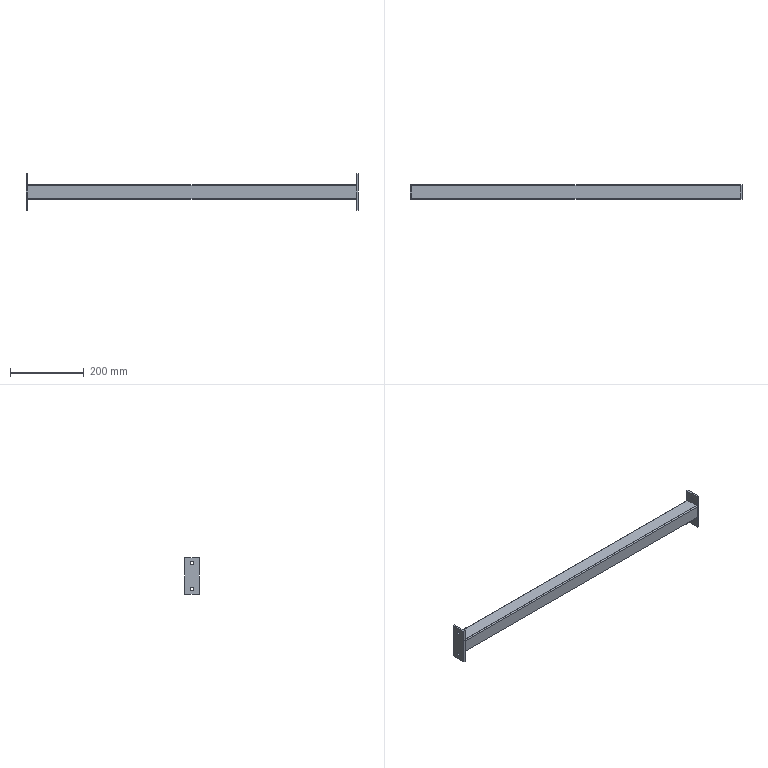Part | SolidWorks | features BaseBody 3 | 3 solids | 38 faces | box 897.45 x 40 x 100 mm | volume 238563 mm3 | plane 22 | cylinder 16 | commonest cylinder face diameters 9 x6 3 x4 6 x4 9.323 x2
STEP:
#1=CARTESIAN_POINT('',(0.,20.,17.));
#2=VERTEX_POINT('',#1);
#3=CARTESIAN_POINT('',(0.,17.,20.));
#4=VERTEX_POINT('',#3);
#5=CARTESIAN_POINT('',(0.,17.,17.));
#6=DIRECTION('',(1.,0.,0.));
#7=DIRECTION('',(0.,0.,-1.));
#8=AXIS2_PLACEMENT_3D('',#5,#6,#7);
#9=CIRCLE('',#8,3.);
#10=EDGE_CURVE('',#2,#4,#9,.T.);
#11=ORIENTED_EDGE('',*,*,#10,.T.);
#12=CARTESIAN_POINT('',(887.45,17.,20.));
#13=VERTEX_POINT('',#12);
#14=CARTESIAN_POINT('',(887.45,17.,20.));
#15=DIRECTION('',(-1.,0.,0.));
#16=VECTOR('',#15,1000.);
#17=LINE('',#14,#16);
#18=EDGE_CURVE('',#13,#4,#17,.T.);
#19=ORIENTED_EDGE('',*,*,#18,.F.);
#20=CARTESIAN_POINT('',(887.45,20.,17.));
#21=VERTEX_POINT('',#20);
#22=CARTESIAN_POINT('',(887.45,17.,17.));
#23=DIRECTION('',(1.,0.,0.));
#24=DIRECTION('',(0.,0.,-1.));
#25=AXIS2_PLACEMENT_3D('',#22,#23,#24);
#26=CIRCLE('',#25,3.);
#27=EDGE_CURVE('',#21,#13,#26,.T.);
#28=ORIENTED_EDGE('',*,*,#27,.F.);
#29=CARTESIAN_POINT('',(887.45,20.,17.));
#30=DIRECTION('',(-1.,0.,0.));
#31=VECTOR('',#30,1000.);
#32=LINE('',#29,#31);
#33=EDGE_CURVE('',#21,#2,#32,.T.);
#34=ORIENTED_EDGE('',*,*,#33,.T.);
#35=EDGE_LOOP('',(#11,#19,#28,#34));
#36=FACE_OUTER_BOUND('',#35,.T.);
#37=CARTESIAN_POINT('',(887.45,17.,17.));
#38=DIRECTION('',(-1.,0.,0.));
#39=DIRECTION('',(0.,0.,1.));
#40=AXIS2_PLACEMENT_3D('',#37,#38,#39);
#41=CYLINDRICAL_SURFACE('',#40,3.);
#42=ADVANCED_FACE('',(#36),#41,.T.);
#43=CARTESIAN_POINT('',(0.,-17.,20.));
#44=VERTEX_POINT('',#43);
#45=CARTESIAN_POINT('',(0.,17.,20.));
#46=DIRECTION('',(0.,-1.,0.));
#47=VECTOR('',#46,1000.);
#48=LINE('',#45,#47);
#49=EDGE_CURVE('',#4,#44,#48,.T.);
#50=ORIENTED_EDGE('',*,*,#49,.T.);
#51=CARTESIAN_POINT('',(887.45,-17.,20.));
#52=VERTEX_POINT('',#51);
#53=CARTESIAN_POINT('',(887.45,-17.,20.));
#54=DIRECTION('',(-1.,0.,0.));
#55=VECTOR('',#54,1000.);
#56=LINE('',#53,#55);
#57=EDGE_CURVE('',#52,#44,#56,.T.);
#58=ORIENTED_EDGE('',*,*,#57,.F.);
#59=CARTESIAN_POINT('',(887.45,17.,20.));
#60=DIRECTION('',(0.,-1.,0.));
#61=VECTOR('',#60,1000.);
#62=LINE('',#59,#61);
#63=EDGE_CURVE('',#13,#52,#62,.T.);
#64=ORIENTED_EDGE('',*,*,#63,.F.);
#65=ORIENTED_EDGE('',*,*,#18,.T.);
#66=EDGE_LOOP('',(#50,#58,#64,#65));
#67=FACE_OUTER_BOUND('',#66,.T.);
#68=CARTESIAN_POINT('',(887.45,17.,20.));
#69=DIRECTION('',(0.,0.,-1.));
#70=DIRECTION('',(0.,1.,0.));
#71=AXIS2_PLACEMENT_3D('',#68,#69,#70);
#72=PLANE('',#71);
#73=ADVANCED_FACE('',(#67),#72,.F.);
#74=CARTESIAN_POINT('',(0.,-20.,17.));
#75=VERTEX_POINT('',#74);
#76=CARTESIAN_POINT('',(0.,-17.,17.));
#77=DIRECTION('',(1.,0.,0.));
#78=DIRECTION('',(0.,0.,-1.));
#79=AXIS2_PLACEMENT_3D('',#76,#77,#78);
#80=CIRCLE('',#79,3.);
#81=EDGE_CURVE('',#44,#75,#80,.T.);
#82=ORIENTED_EDGE('',*,*,#81,.T.);
#83=CARTESIAN_POINT('',(887.45,-20.,17.));
#84=VERTEX_POINT('',#83);
#85=CARTESIAN_POINT('',(887.45,-20.,17.));
#86=DIRECTION('',(-1.,0.,0.));
#87=VECTOR('',#86,1000.);
#88=LINE('',#85,#87);
#89=EDGE_CURVE('',#84,#75,#88,.T.);
#90=ORIENTED_EDGE('',*,*,#89,.F.);
#91=CARTESIAN_POINT('',(887.45,-17.,17.));
#92=DIRECTION('',(1.,0.,0.));
#93=DIRECTION('',(0.,0.,-1.));
#94=AXIS2_PLACEMENT_3D('',#91,#92,#93);
#95=CIRCLE('',#94,3.);
#96=EDGE_CURVE('',#52,#84,#95,.T.);
#97=ORIENTED_EDGE('',*,*,#96,.F.);
#98=ORIENTED_EDGE('',*,*,#57,.T.);
#99=EDGE_LOOP('',(#82,#90,#97,#98));
#100=FACE_OUTER_BOUND('',#99,.T.);
#101=CARTESIAN_POINT('',(887.45,-17.,17.));
#102=DIRECTION('',(-1.,0.,0.));
#103=DIRECTION('',(0.,0.,1.));
#104=AXIS2_PLACEMENT_3D('',#101,#102,#103);
#105=CYLINDRICAL_SURFACE('',#104,3.);
#106=ADVANCED_FACE('',(#100),#105,.T.);
#107=CARTESIAN_POINT('',(0.,-20.,-17.));
#108=VERTEX_POINT('',#107);
#109=CARTESIAN_POINT('',(0.,-20.,-17.));
#110=DIRECTION('',(0.,0.,-1.));
#111=VECTOR('',#110,1000.);
#112=LINE('',#109,#111);
#113=EDGE_CURVE('',#75,#108,#112,.T.);
#114=ORIENTED_EDGE('',*,*,#113,.T.);
#115=CARTESIAN_POINT('',(887.45,-20.,-17.));
#116=VERTEX_POINT('',#115);
#117=CARTESIAN_POINT('',(887.45,-20.,-17.));
#118=DIRECTION('',(-1.,0.,0.));
#119=VECTOR('',#118,1000.);
#120=LINE('',#117,#119);
#121=EDGE_CURVE('',#116,#108,#120,.T.);
#122=ORIENTED_EDGE('',*,*,#121,.F.);
#123=CARTESIAN_POINT('',(887.45,-20.,-17.));
#124=DIRECTION('',(0.,0.,-1.));
#125=VECTOR('',#124,1000.);
#126=LINE('',#123,#125);
#127=EDGE_CURVE('',#84,#116,#126,.T.);
#128=ORIENTED_EDGE('',*,*,#127,.F.);
#129=ORIENTED_EDGE('',*,*,#89,.T.);
#130=EDGE_LOOP('',(#114,#122,#128,#129));
#131=FACE_OUTER_BOUND('',#130,.T.);
#132=CARTESIAN_POINT('',(887.45,-20.,-17.));
#133=DIRECTION('',(0.,1.,0.));
#134=DIRECTION('',(0.,0.,1.));
#135=AXIS2_PLACEMENT_3D('',#132,#133,#134);
#136=PLANE('',#135);
#137=ADVANCED_FACE('',(#131),#136,.F.);
#138=CARTESIAN_POINT('',(0.,-17.,-20.));
#139=VERTEX_POINT('',#138);
#140=CARTESIAN_POINT('',(0.,-17.,-17.));
#141=DIRECTION('',(1.,0.,0.));
#142=DIRECTION('',(0.,0.,-1.));
#143=AXIS2_PLACEMENT_3D('',#140,#141,#142);
#144=CIRCLE('',#143,3.);
#145=EDGE_CURVE('',#108,#139,#144,.T.);
#146=ORIENTED_EDGE('',*,*,#145,.T.);
#147=CARTESIAN_POINT('',(887.45,-17.,-20.));
#148=VERTEX_POINT('',#147);
#149=CARTESIAN_POINT('',(887.45,-17.,-20.));
#150=DIRECTION('',(-1.,0.,0.));
#151=VECTOR('',#150,1000.);
#152=LINE('',#149,#151);
#153=EDGE_CURVE('',#148,#139,#152,.T.);
#154=ORIENTED_EDGE('',*,*,#153,.F.);
#155=CARTESIAN_POINT('',(887.45,-17.,-17.));
#156=DIRECTION('',(1.,0.,0.));
#157=DIRECTION('',(0.,0.,-1.));
#158=AXIS2_PLACEMENT_3D('',#155,#156,#157);
#159=CIRCLE('',#158,3.);
#160=EDGE_CURVE('',#116,#148,#159,.T.);
#161=ORIENTED_EDGE('',*,*,#160,.F.);
#162=ORIENTED_EDGE('',*,*,#121,.T.);
#163=EDGE_LOOP('',(#146,#154,#161,#162));
#164=FACE_OUTER_BOUND('',#163,.T.);
#165=CARTESIAN_POINT('',(887.45,-17.,-17.));
#166=DIRECTION('',(-1.,0.,0.));
#167=DIRECTION('',(0.,0.,1.));
#168=AXIS2_PLACEMENT_3D('',#165,#166,#167);
#169=CYLINDRICAL_SURFACE('',#168,3.);
#170=ADVANCED_FACE('',(#164),#169,.T.);
#171=CARTESIAN_POINT('',(0.,17.,-20.));
#172=VERTEX_POINT('',#171);
#173=CARTESIAN_POINT('',(0.,-17.,-20.));
#174=DIRECTION('',(0.,1.,0.));
#175=VECTOR('',#174,1000.);
#176=LINE('',#173,#175);
#177=EDGE_CURVE('',#139,#172,#176,.T.);
#178=ORIENTED_EDGE('',*,*,#177,.T.);
#179=CARTESIAN_POINT('',(887.45,17.,-20.));
#180=VERTEX_POINT('',#179);
#181=CARTESIAN_POINT('',(887.45,17.,-20.));
#182=DIRECTION('',(-1.,0.,0.));
#183=VECTOR('',#182,1000.);
#184=LINE('',#181,#183);
#185=EDGE_CURVE('',#180,#172,#184,.T.);
#186=ORIENTED_EDGE('',*,*,#185,.F.);
#187=CARTESIAN_POINT('',(887.45,-17.,-20.));
#188=DIRECTION('',(0.,1.,0.));
#189=VECTOR('',#188,1000.);
#190=LINE('',#187,#189);
#191=EDGE_CURVE('',#148,#180,#190,.T.);
#192=ORIENTED_EDGE('',*,*,#191,.F.);
#193=ORIENTED_EDGE('',*,*,#153,.T.);
#194=EDGE_LOOP('',(#178,#186,#192,#193));
#195=FACE_OUTER_BOUND('',#194,.T.);
#196=CARTESIAN_POINT('',(887.45,-17.,-20.));
#197=DIRECTION('',(0.,0.,1.));
#198=DIRECTION('',(0.,-1.,0.));
#199=AXIS2_PLACEMENT_3D('',#196,#197,#198);
#200=PLANE('',#199);
#201=ADVANCED_FACE('',(#195),#200,.F.);
#202=CARTESIAN_POINT('',(0.,20.,-17.));
#203=VERTEX_POINT('',#202);
#204=CARTESIAN_POINT('',(0.,17.,-17.));
#205=DIRECTION('',(1.,0.,0.));
#206=DIRECTION('',(0.,0.,-1.));
#207=AXIS2_PLACEMENT_3D('',#204,#205,#206);
#208=CIRCLE('',#207,3.);
#209=EDGE_CURVE('',#172,#203,#208,.T.);
#210=ORIENTED_EDGE('',*,*,#209,.T.);
#211=CARTESIAN_POINT('',(887.45,20.,-17.));
#212=VERTEX_POINT('',#211);
#213=CARTESIAN_POINT('',(887.45,20.,-17.));
#214=DIRECTION('',(-1.,0.,0.));
#215=VECTOR('',#214,1000.);
#216=LINE('',#213,#215);
#217=EDGE_CURVE('',#212,#203,#216,.T.);
#218=ORIENTED_EDGE('',*,*,#217,.F.);
#219=CARTESIAN_POINT('',(887.45,17.,-17.));
#220=DIRECTION('',(1.,0.,0.));
#221=DIRECTION('',(0.,0.,-1.));
#222=AXIS2_PLACEMENT_3D('',#219,#220,#221);
#223=CIRCLE('',#222,3.);
#224=EDGE_CURVE('',#180,#212,#223,.T.);
#225=ORIENTED_EDGE('',*,*,#224,.F.);
#226=ORIENTED_EDGE('',*,*,#185,.T.);
#227=EDGE_LOOP('',(#210,#218,#225,#226));
#228=FACE_OUTER_BOUND('',#227,.T.);
#229=CARTESIAN_POINT('',(887.45,17.,-17.));
#230=DIRECTION('',(-1.,0.,0.));
#231=DIRECTION('',(0.,0.,1.));
#232=AXIS2_PLACEMENT_3D('',#229,#230,#231);
#233=CYLINDRICAL_SURFACE('',#232,3.);
#234=ADVANCED_FACE('',(#228),#233,.T.);
#235=CARTESIAN_POINT('',(0.,-17.,18.5));
#236=VERTEX_POINT('',#235);
#237=CARTESIAN_POINT('',(0.,-18.5,17.));
#238=VERTEX_POINT('',#237);
#239=CARTESIAN_POINT('',(0.,-17.,17.));
#240=DIRECTION('',(1.,0.,0.));
#241=DIRECTION('',(0.,0.,-1.));
#242=AXIS2_PLACEMENT_3D('',#239,#240,#241);
#243=CIRCLE('',#242,1.5);
#244=EDGE_CURVE('',#236,#238,#243,.T.);
#245=ORIENTED_EDGE('',*,*,#244,.F.);
#246=CARTESIAN_POINT('',(887.45,-17.,18.5));
#247=VERTEX_POINT('',#246);
#248=CARTESIAN_POINT('',(887.45,-17.,18.5));
#249=DIRECTION('',(-1.,0.,0.));
#250=VECTOR('',#249,1000.);
#251=LINE('',#248,#250);
#252=EDGE_CURVE('',#247,#236,#251,.T.);
#253=ORIENTED_EDGE('',*,*,#252,.F.);
#254=CARTESIAN_POINT('',(887.45,-18.5,17.));
#255=VERTEX_POINT('',#254);
#256=CARTESIAN_POINT('',(887.45,-17.,17.));
#257=DIRECTION('',(1.,0.,0.));
#258=DIRECTION('',(0.,0.,-1.));
#259=AXIS2_PLACEMENT_3D('',#256,#257,#258);
#260=CIRCLE('',#259,1.5);
#261=EDGE_CURVE('',#247,#255,#260,.T.);
#262=ORIENTED_EDGE('',*,*,#261,.T.);
#263=CARTESIAN_POINT('',(887.45,-18.5,17.));
#264=DIRECTION('',(-1.,0.,0.));
#265=VECTOR('',#264,1000.);
#266=LINE('',#263,#265);
#267=EDGE_CURVE('',#255,#238,#266,.T.);
#268=ORIENTED_EDGE('',*,*,#267,.T.);
#269=EDGE_LOOP('',(#245,#253,#262,#268));
#270=FACE_OUTER_BOUND('',#269,.T.);
#271=CARTESIAN_POINT('',(887.45,-17.,17.));
#272=DIRECTION('',(-1.,0.,0.));
#273=DIRECTION('',(0.,0.,1.));
#274=AXIS2_PLACEMENT_3D('',#271,#272,#273);
#275=CYLINDRICAL_SURFACE('',#274,1.5);
#276=ADVANCED_FACE('',(#270),#275,.F.);
#277=CARTESIAN_POINT('',(0.,17.,18.5));
#278=VERTEX_POINT('',#277);
#279=CARTESIAN_POINT('',(0.,17.,18.5));
#280=DIRECTION('',(0.,-1.,0.));
#281=VECTOR('',#280,1000.);
#282=LINE('',#279,#281);
#283=EDGE_CURVE('',#278,#236,#282,.T.);
#284=ORIENTED_EDGE('',*,*,#283,.F.);
#285=CARTESIAN_POINT('',(887.45,17.,18.5));
#286=VERTEX_POINT('',#285);
#287=CARTESIAN_POINT('',(887.45,17.,18.5));
#288=DIRECTION('',(-1.,0.,0.));
#289=VECTOR('',#288,1000.);
#290=LINE('',#287,#289);
#291=EDGE_CURVE('',#286,#278,#290,.T.);
#292=ORIENTED_EDGE('',*,*,#291,.F.);
#293=CARTESIAN_POINT('',(887.45,17.,18.5));
#294=DIRECTION('',(0.,-1.,0.));
#295=VECTOR('',#294,1000.);
#296=LINE('',#293,#295);
#297=EDGE_CURVE('',#286,#247,#296,.T.);
#298=ORIENTED_EDGE('',*,*,#297,.T.);
#299=ORIENTED_EDGE('',*,*,#252,.T.);
#300=EDGE_LOOP('',(#284,#292,#298,#299));
#301=FACE_OUTER_BOUND('',#300,.T.);
#302=CARTESIAN_POINT('',(887.45,17.,18.5));
#303=DIRECTION('',(0.,0.,-1.));
#304=DIRECTION('',(0.,1.,0.));
#305=AXIS2_PLACEMENT_3D('',#302,#303,#304);
#306=PLANE('',#305);
#307=ADVANCED_FACE('',(#301),#306,.T.);
#308=CARTESIAN_POINT('',(0.,18.5,17.));
#309=VERTEX_POINT('',#308);
#310=CARTESIAN_POINT('',(0.,17.,17.));
#311=DIRECTION('',(1.,0.,0.));
#312=DIRECTION('',(0.,0.,-1.));
#313=AXIS2_PLACEMENT_3D('',#310,#311,#312);
#314=CIRCLE('',#313,1.5);
#315=EDGE_CURVE('',#309,#278,#314,.T.);
#316=ORIENTED_EDGE('',*,*,#315,.F.);
#317=CARTESIAN_POINT('',(887.45,18.5,17.));
#318=VERTEX_POINT('',#317);
#319=CARTESIAN_POINT('',(887.45,18.5,17.));
#320=DIRECTION('',(-1.,0.,0.));
#321=VECTOR('',#320,1000.);
#322=LINE('',#319,#321);
#323=EDGE_CURVE('',#318,#309,#322,.T.);
#324=ORIENTED_EDGE('',*,*,#323,.F.);
#325=CARTESIAN_POINT('',(887.45,17.,17.));
#326=DIRECTION('',(1.,0.,0.));
#327=DIRECTION('',(0.,0.,-1.));
#328=AXIS2_PLACEMENT_3D('',#325,#326,#327);
#329=CIRCLE('',#328,1.5);
#330=EDGE_CURVE('',#318,#286,#329,.T.);
#331=ORIENTED_EDGE('',*,*,#330,.T.);
#332=ORIENTED_EDGE('',*,*,#291,.T.);
#333=EDGE_LOOP('',(#316,#324,#331,#332));
#334=FACE_OUTER_BOUND('',#333,.T.);
#335=CARTESIAN_POINT('',(887.45,17.,17.));
#336=DIRECTION('',(-1.,0.,0.));
#337=DIRECTION('',(0.,0.,1.));
#338=AXIS2_PLACEMENT_3D('',#335,#336,#337);
#339=CYLINDRICAL_SURFACE('',#338,1.5);
#340=ADVANCED_FACE('',(#334),#339,.F.);
#341=CARTESIAN_POINT('',(0.,18.5,-17.));
#342=VERTEX_POINT('',#341);
#343=CARTESIAN_POINT('',(0.,18.5,17.));
#344=DIRECTION('',(0.,0.,1.));
#345=VECTOR('',#344,1000.);
#346=LINE('',#343,#345);
#347=EDGE_CURVE('',#342,#309,#346,.T.);
#348=ORIENTED_EDGE('',*,*,#347,.F.);
#349=CARTESIAN_POINT('',(887.45,18.5,-17.));
#350=VERTEX_POINT('',#349);
#351=CARTESIAN_POINT('',(887.45,18.5,-17.));
#352=DIRECTION('',(-1.,0.,0.));
#353=VECTOR('',#352,1000.);
#354=LINE('',#351,#353);
#355=EDGE_CURVE('',#350,#342,#354,.T.);
#356=ORIENTED_EDGE('',*,*,#355,.F.);
#357=CARTESIAN_POINT('',(887.45,18.5,17.));
#358=DIRECTION('',(0.,0.,1.));
#359=VECTOR('',#358,1000.);
#360=LINE('',#357,#359);
#361=EDGE_CURVE('',#350,#318,#360,.T.);
#362=ORIENTED_EDGE('',*,*,#361,.T.);
#363=ORIENTED_EDGE('',*,*,#323,.T.);
#364=EDGE_LOOP('',(#348,#356,#362,#363));
#365=FACE_OUTER_BOUND('',#364,.T.);
#366=CARTESIAN_POINT('',(887.45,18.5,17.));
#367=DIRECTION('',(0.,-1.,0.));
#368=DIRECTION('',(0.,0.,-1.));
#369=AXIS2_PLACEMENT_3D('',#366,#367,#368);
#370=PLANE('',#369);
#371=ADVANCED_FACE('',(#365),#370,.T.);
#372=CARTESIAN_POINT('',(0.,17.,-18.5));
#373=VERTEX_POINT('',#372);
#374=CARTESIAN_POINT('',(0.,17.,-17.));
#375=DIRECTION('',(1.,0.,0.));
#376=DIRECTION('',(0.,0.,-1.));
#377=AXIS2_PLACEMENT_3D('',#374,#375,#376);
#378=CIRCLE('',#377,1.5);
#379=EDGE_CURVE('',#373,#342,#378,.T.);
#380=ORIENTED_EDGE('',*,*,#379,.F.);
#381=CARTESIAN_POINT('',(887.45,17.,-18.5));
#382=VERTEX_POINT('',#381);
#383=CARTESIAN_POINT('',(887.45,17.,-18.5));
#384=DIRECTION('',(-1.,0.,0.));
#385=VECTOR('',#384,1000.);
#386=LINE('',#383,#385);
#387=EDGE_CURVE('',#382,#373,#386,.T.);
#388=ORIENTED_EDGE('',*,*,#387,.F.);
#389=CARTESIAN_POINT('',(887.45,17.,-17.));
#390=DIRECTION('',(1.,0.,0.));
#391=DIRECTION('',(0.,0.,-1.));
#392=AXIS2_PLACEMENT_3D('',#389,#390,#391);
#393=CIRCLE('',#392,1.5);
#394=EDGE_CURVE('',#382,#350,#393,.T.);
#395=ORIENTED_EDGE('',*,*,#394,.T.);
#396=ORIENTED_EDGE('',*,*,#355,.T.);
#397=EDGE_LOOP('',(#380,#388,#395,#396));
#398=FACE_OUTER_BOUND('',#397,.T.);
#399=CARTESIAN_POINT('',(887.45,17.,-17.));
#400=DIRECTION('',(-1.,0.,0.));
#401=DIRECTION('',(0.,0.,1.));
#402=AXIS2_PLACEMENT_3D('',#399,#400,#401);
#403=CYLINDRICAL_SURFACE('',#402,1.5);
#404=ADVANCED_FACE('',(#398),#403,.F.);
#405=CARTESIAN_POINT('',(0.,-17.,-18.5));
#406=VERTEX_POINT('',#405);
#407=CARTESIAN_POINT('',(0.,-17.,-18.5));
#408=DIRECTION('',(0.,1.,0.));
#409=VECTOR('',#408,1000.);
#410=LINE('',#407,#409);
#411=EDGE_CURVE('',#406,#373,#410,.T.);
#412=ORIENTED_EDGE('',*,*,#411,.F.);
#413=CARTESIAN_POINT('',(887.45,-17.,-18.5));
#414=VERTEX_POINT('',#413);
#415=CARTESIAN_POINT('',(887.45,-17.,-18.5));
#416=DIRECTION('',(-1.,0.,0.));
#417=VECTOR('',#416,1000.);
#418=LINE('',#415,#417);
#419=EDGE_CURVE('',#414,#406,#418,.T.);
#420=ORIENTED_EDGE('',*,*,#419,.F.);
#421=CARTESIAN_POINT('',(887.45,-17.,-18.5));
#422=DIRECTION('',(0.,1.,0.));
#423=VECTOR('',#422,1000.);
#424=LINE('',#421,#423);
#425=EDGE_CURVE('',#414,#382,#424,.T.);
#426=ORIENTED_EDGE('',*,*,#425,.T.);
#427=ORIENTED_EDGE('',*,*,#387,.T.);
#428=EDGE_LOOP('',(#412,#420,#426,#427));
#429=FACE_OUTER_BOUND('',#428,.T.);
#430=CARTESIAN_POINT('',(887.45,-17.,-18.5));
#431=DIRECTION('',(0.,0.,1.));
#432=DIRECTION('',(0.,-1.,0.));
#433=AXIS2_PLACEMENT_3D('',#430,#431,#432);
#434=PLANE('',#433);
#435=ADVANCED_FACE('',(#429),#434,.T.);
#436=CARTESIAN_POINT('',(0.,-18.5,-17.));
#437=VERTEX_POINT('',#436);
#438=CARTESIAN_POINT('',(0.,-17.,-17.));
#439=DIRECTION('',(1.,0.,0.));
#440=DIRECTION('',(0.,0.,-1.));
#441=AXIS2_PLACEMENT_3D('',#438,#439,#440);
#442=CIRCLE('',#441,1.5);
#443=EDGE_CURVE('',#437,#406,#442,.T.);
#444=ORIENTED_EDGE('',*,*,#443,.F.);
#445=CARTESIAN_POINT('',(887.45,-18.5,-17.));
#446=VERTEX_POINT('',#445);
#447=CARTESIAN_POINT('',(887.45,-18.5,-17.));
#448=DIRECTION('',(-1.,0.,0.));
#449=VECTOR('',#448,1000.);
#450=LINE('',#447,#449);
#451=EDGE_CURVE('',#446,#437,#450,.T.);
#452=ORIENTED_EDGE('',*,*,#451,.F.);
#453=CARTESIAN_POINT('',(887.45,-17.,-17.));
#454=DIRECTION('',(1.,0.,0.));
#455=DIRECTION('',(0.,0.,-1.));
#456=AXIS2_PLACEMENT_3D('',#453,#454,#455);
#457=CIRCLE('',#456,1.5);
#458=EDGE_CURVE('',#446,#414,#457,.T.);
#459=ORIENTED_EDGE('',*,*,#458,.T.);
#460=ORIENTED_EDGE('',*,*,#419,.T.);
#461=EDGE_LOOP('',(#444,#452,#459,#460));
#462=FACE_OUTER_BOUND('',#461,.T.);
#463=CARTESIAN_POINT('',(887.45,-17.,-17.));
#464=DIRECTION('',(-1.,0.,0.));
#465=DIRECTION('',(0.,0.,1.));
#466=AXIS2_PLACEMENT_3D('',#463,#464,#465);
#467=CYLINDRICAL_SURFACE('',#466,1.5);
#468=ADVANCED_FACE('',(#462),#467,.F.);
#469=CARTESIAN_POINT('',(0.,-18.5,-17.));
#470=DIRECTION('',(0.,0.,-1.));
#471=VECTOR('',#470,1000.);
#472=LINE('',#469,#471);
#473=EDGE_CURVE('',#238,#437,#472,.T.);
#474=ORIENTED_EDGE('',*,*,#473,.F.);
#475=ORIENTED_EDGE('',*,*,#267,.F.);
#476=CARTESIAN_POINT('',(887.45,-18.5,-17.));
#477=DIRECTION('',(0.,0.,-1.));
#478=VECTOR('',#477,1000.);
#479=LINE('',#476,#478);
#480=EDGE_CURVE('',#255,#446,#479,.T.);
#481=ORIENTED_EDGE('',*,*,#480,.T.);
#482=ORIENTED_EDGE('',*,*,#451,.T.);
#483=EDGE_LOOP('',(#474,#475,#481,#482));
#484=FACE_OUTER_BOUND('',#483,.T.);
#485=CARTESIAN_POINT('',(887.45,-18.5,-17.));
#486=DIRECTION('',(0.,1.,0.));
#487=DIRECTION('',(0.,0.,1.));
#488=AXIS2_PLACEMENT_3D('',#485,#486,#487);
#489=PLANE('',#488);
#490=ADVANCED_FACE('',(#484),#489,.T.);
#491=CARTESIAN_POINT('',(0.,20.,17.));
#492=DIRECTION('',(0.,0.,1.));
#493=VECTOR('',#492,1000.);
#494=LINE('',#491,#493);
#495=EDGE_CURVE('',#203,#2,#494,.T.);
#496=ORIENTED_EDGE('',*,*,#495,.T.);
#497=ORIENTED_EDGE('',*,*,#33,.F.);
#498=CARTESIAN_POINT('',(887.45,20.,17.));
#499=DIRECTION('',(0.,0.,1.));
#500=VECTOR('',#499,1000.);
#501=LINE('',#498,#500);
#502=EDGE_CURVE('',#212,#21,#501,.T.);
#503=ORIENTED_EDGE('',*,*,#502,.F.);
#504=ORIENTED_EDGE('',*,*,#217,.T.);
#505=EDGE_LOOP('',(#496,#497,#503,#504));
#506=FACE_OUTER_BOUND('',#505,.T.);
#507=CARTESIAN_POINT('',(887.45,20.,17.));
#508=DIRECTION('',(0.,-1.,0.));
#509=DIRECTION('',(0.,0.,-1.));
#510=AXIS2_PLACEMENT_3D('',#507,#508,#509);
#511=PLANE('',#510);
#512=ADVANCED_FACE('',(#506),#511,.F.);
#513=ORIENTED_EDGE('',*,*,#261,.F.);
#514=ORIENTED_EDGE('',*,*,#297,.F.);
#515=ORIENTED_EDGE('',*,*,#330,.F.);
#516=ORIENTED_EDGE('',*,*,#361,.F.);
#517=ORIENTED_EDGE('',*,*,#394,.F.);
#518=ORIENTED_EDGE('',*,*,#425,.F.);
#519=ORIENTED_EDGE('',*,*,#458,.F.);
#520=ORIENTED_EDGE('',*,*,#480,.F.);
#521=EDGE_LOOP('',(#513,#514,#515,#516,#517,#518,#519,#520));
#522=FACE_BOUND('',#521,.T.);
#523=ORIENTED_EDGE('',*,*,#27,.T.);
#524=ORIENTED_EDGE('',*,*,#63,.T.);
#525=ORIENTED_EDGE('',*,*,#96,.T.);
#526=ORIENTED_EDGE('',*,*,#127,.T.);
#527=ORIENTED_EDGE('',*,*,#160,.T.);
#528=ORIENTED_EDGE('',*,*,#191,.T.);
#529=ORIENTED_EDGE('',*,*,#224,.T.);
#530=ORIENTED_EDGE('',*,*,#502,.T.);
#531=EDGE_LOOP('',(#523,#524,#525,#526,#527,#528,#529,#530));
#532=FACE_OUTER_BOUND('',#531,.T.);
#533=CARTESIAN_POINT('',(887.45,17.,17.));
#534=DIRECTION('',(1.,0.,0.));
#535=DIRECTION('',(0.,0.,-1.));
#536=AXIS2_PLACEMENT_3D('',#533,#534,#535);
#537=PLANE('',#536);
#538=ADVANCED_FACE('',(#522,#532),#537,.T.);
#539=ORIENTED_EDGE('',*,*,#244,.T.);
#540=ORIENTED_EDGE('',*,*,#473,.T.);
#541=ORIENTED_EDGE('',*,*,#443,.T.);
#542=ORIENTED_EDGE('',*,*,#411,.T.);
#543=ORIENTED_EDGE('',*,*,#379,.T.);
#544=ORIENTED_EDGE('',*,*,#347,.T.);
#545=ORIENTED_EDGE('',*,*,#315,.T.);
#546=ORIENTED_EDGE('',*,*,#283,.T.);
#547=EDGE_LOOP('',(#539,#540,#541,#542,#543,#544,#545,#546));
#548=FACE_BOUND('',#547,.T.);
#549=ORIENTED_EDGE('',*,*,#10,.F.);
#550=ORIENTED_EDGE('',*,*,#495,.F.);
#551=ORIENTED_EDGE('',*,*,#209,.F.);
#552=ORIENTED_EDGE('',*,*,#177,.F.);
#553=ORIENTED_EDGE('',*,*,#145,.F.);
#554=ORIENTED_EDGE('',*,*,#113,.F.);
#555=ORIENTED_EDGE('',*,*,#81,.F.);
#556=ORIENTED_EDGE('',*,*,#49,.F.);
#557=EDGE_LOOP('',(#549,#550,#551,#552,#553,#554,#555,#556));
#558=FACE_OUTER_BOUND('',#557,.T.);
#559=CARTESIAN_POINT('',(0.,17.,17.));
#560=DIRECTION('',(1.,0.,0.));
#561=DIRECTION('',(0.,0.,-1.));
#562=AXIS2_PLACEMENT_3D('',#559,#560,#561);
#563=PLANE('',#562);
#564=ADVANCED_FACE('',(#548,#558),#563,.F.);
#565=CLOSED_SHELL('',(#42,#73,#106,#137,#170,#201,#234,#276,#307,#340,#371,#404,#435,#468,#490,#512,#538,#564));
#566=MANIFOLD_SOLID_BREP('',#565);
#567=CARTESIAN_POINT('',(892.45,0.,39.5));
#568=VERTEX_POINT('',#567);
#569=CARTESIAN_POINT('',(892.45,0.,30.5));
#570=VERTEX_POINT('',#569);
#571=CARTESIAN_POINT('',(892.45,0.,35.));
#572=DIRECTION('',(1.,0.,0.));
#573=DIRECTION('',(0.,0.,-1.));
#574=AXIS2_PLACEMENT_3D('',#571,#572,#573);
#575=CIRCLE('',#574,4.5);
#576=EDGE_CURVE('',#568,#570,#575,.T.);
#577=ORIENTED_EDGE('',*,*,#576,.T.);
#578=CARTESIAN_POINT('',(887.45,0.,30.5));
#579=VERTEX_POINT('',#578);
#580=CARTESIAN_POINT('',(892.45,0.,30.5));
#581=DIRECTION('',(-1.,0.,0.));
#582=VECTOR('',#581,1000.);
#583=LINE('',#580,#582);
#584=EDGE_CURVE('',#570,#579,#583,.T.);
#585=ORIENTED_EDGE('',*,*,#584,.T.);
#586=CARTESIAN_POINT('',(887.45,0.,39.5));
#587=VERTEX_POINT('',#586);
#588=CARTESIAN_POINT('',(887.45,0.,35.));
#589=DIRECTION('',(1.,0.,0.));
#590=DIRECTION('',(0.,0.,-1.));
#591=AXIS2_PLACEMENT_3D('',#588,#589,#590);
#592=CIRCLE('',#591,4.5);
#593=EDGE_CURVE('',#587,#579,#592,.T.);
#594=ORIENTED_EDGE('',*,*,#593,.F.);
#595=CARTESIAN_POINT('',(892.45,0.,39.5));
#596=DIRECTION('',(-1.,0.,0.));
#597=VECTOR('',#596,1000.);
#598=LINE('',#595,#597);
#599=EDGE_CURVE('',#568,#587,#598,.T.);
#600=ORIENTED_EDGE('',*,*,#599,.F.);
#601=EDGE_LOOP('',(#577,#585,#594,#600));
#602=FACE_OUTER_BOUND('',#601,.T.);
#603=CARTESIAN_POINT('',(892.45,0.,35.));
#604=DIRECTION('',(-1.,0.,0.));
#605=DIRECTION('',(0.,0.,1.));
#606=AXIS2_PLACEMENT_3D('',#603,#604,#605);
#607=CYLINDRICAL_SURFACE('',#606,4.5);
#608=ADVANCED_FACE('',(#602),#607,.F.);
#609=CARTESIAN_POINT('',(892.45,0.,-30.5));
#610=VERTEX_POINT('',#609);
#611=CARTESIAN_POINT('',(892.45,0.,-39.5));
#612=VERTEX_POINT('',#611);
#613=CARTESIAN_POINT('',(892.45,0.,-35.));
#614=DIRECTION('',(1.,0.,0.));
#615=DIRECTION('',(0.,0.,-1.));
#616=AXIS2_PLACEMENT_3D('',#613,#614,#615);
#617=CIRCLE('',#616,4.5);
#618=EDGE_CURVE('',#610,#612,#617,.T.);
#619=ORIENTED_EDGE('',*,*,#618,.T.);
#620=CARTESIAN_POINT('',(887.45,0.,-39.5));
#621=VERTEX_POINT('',#620);
#622=CARTESIAN_POINT('',(892.45,0.,-39.5));
#623=DIRECTION('',(-1.,0.,0.));
#624=VECTOR('',#623,1000.);
#625=LINE('',#622,#624);
#626=EDGE_CURVE('',#612,#621,#625,.T.);
#627=ORIENTED_EDGE('',*,*,#626,.T.);
#628=CARTESIAN_POINT('',(887.45,0.,-30.5));
#629=VERTEX_POINT('',#628);
#630=CARTESIAN_POINT('',(887.45,0.,-35.));
#631=DIRECTION('',(1.,0.,0.));
#632=DIRECTION('',(0.,0.,-1.));
#633=AXIS2_PLACEMENT_3D('',#630,#631,#632);
#634=CIRCLE('',#633,4.5);
#635=EDGE_CURVE('',#629,#621,#634,.T.);
#636=ORIENTED_EDGE('',*,*,#635,.F.);
#637=CARTESIAN_POINT('',(892.45,0.,-30.5));
#638=DIRECTION('',(-1.,0.,0.));
#639=VECTOR('',#638,1000.);
#640=LINE('',#637,#639);
#641=EDGE_CURVE('',#610,#629,#640,.T.);
#642=ORIENTED_EDGE('',*,*,#641,.F.);
#643=EDGE_LOOP('',(#619,#627,#636,#642));
#644=FACE_OUTER_BOUND('',#643,.T.);
#645=CARTESIAN_POINT('',(892.45,0.,-35.));
#646=DIRECTION('',(-1.,0.,0.));
#647=DIRECTION('',(0.,0.,1.));
#648=AXIS2_PLACEMENT_3D('',#645,#646,#647);
#649=CYLINDRICAL_SURFACE('',#648,4.5);
#650=ADVANCED_FACE('',(#644),#649,.F.);
#651=CARTESIAN_POINT('',(892.45,-20.,-50.));
#652=VERTEX_POINT('',#651);
#653=CARTESIAN_POINT('',(892.45,20.,-50.));
#654=VERTEX_POINT('',#653);
#655=CARTESIAN_POINT('',(892.45,-20.,-50.));
#656=DIRECTION('',(0.,1.,0.));
#657=VECTOR('',#656,1000.);
#658=LINE('',#655,#657);
#659=EDGE_CURVE('',#652,#654,#658,.T.);
#660=ORIENTED_EDGE('',*,*,#659,.T.);
#661=CARTESIAN_POINT('',(892.45,20.,50.));
#662=VERTEX_POINT('',#661);
#663=CARTESIAN_POINT('',(892.45,20.,50.));
#664=DIRECTION('',(0.,0.,1.));
#665=VECTOR('',#664,1000.);
#666=LINE('',#663,#665);
#667=EDGE_CURVE('',#654,#662,#666,.T.);
#668=ORIENTED_EDGE('',*,*,#667,.T.);
#669=CARTESIAN_POINT('',(892.45,-20.,50.));
#670=VERTEX_POINT('',#669);
#671=CARTESIAN_POINT('',(892.45,-20.,50.));
#672=DIRECTION('',(0.,-1.,0.));
#673=VECTOR('',#672,1000.);
#674=LINE('',#671,#673);
#675=EDGE_CURVE('',#662,#670,#674,.T.);
#676=ORIENTED_EDGE('',*,*,#675,.T.);
#677=CARTESIAN_POINT('',(892.45,-20.,50.));
#678=DIRECTION('',(0.,0.,-1.));
#679=VECTOR('',#678,1000.);
#680=LINE('',#677,#679);
#681=EDGE_CURVE('',#670,#652,#680,.T.);
#682=ORIENTED_EDGE('',*,*,#681,.T.);
#683=EDGE_LOOP('',(#660,#668,#676,#682));
#684=FACE_OUTER_BOUND('',#683,.T.);
#685=ORIENTED_EDGE('',*,*,#618,.F.);
#686=CARTESIAN_POINT('',(892.45,0.,-35.));
#687=DIRECTION('',(1.,0.,0.));
#688=DIRECTION('',(0.,0.,-1.));
#689=AXIS2_PLACEMENT_3D('',#686,#687,#688);
#690=CIRCLE('',#689,4.5);
#691=EDGE_CURVE('',#612,#610,#690,.T.);
#692=ORIENTED_EDGE('',*,*,#691,.F.);
#693=EDGE_LOOP('',(#685,#692));
#694=FACE_BOUND('',#693,.T.);
#695=ORIENTED_EDGE('',*,*,#576,.F.);
#696=CARTESIAN_POINT('',(892.45,0.,35.));
#697=DIRECTION('',(1.,0.,0.));
#698=DIRECTION('',(0.,0.,-1.));
#699=AXIS2_PLACEMENT_3D('',#696,#697,#698);
#700=CIRCLE('',#699,4.5);
#701=EDGE_CURVE('',#570,#568,#700,.T.);
#702=ORIENTED_EDGE('',*,*,#701,.F.);
#703=EDGE_LOOP('',(#695,#702));
#704=FACE_BOUND('',#703,.T.);
#705=CARTESIAN_POINT('',(892.45,0.,0.));
#706=DIRECTION('',(-1.,0.,0.));
#707=DIRECTION('',(0.,0.,1.));
#708=AXIS2_PLACEMENT_3D('',#705,#706,#707);
#709=PLANE('',#708);
#710=ADVANCED_FACE('',(#684,#694,#704),#709,.F.);
#711=ORIENTED_EDGE('',*,*,#635,.T.);
#712=CARTESIAN_POINT('',(887.45,0.,-35.));
#713=DIRECTION('',(1.,0.,0.));
#714=DIRECTION('',(0.,0.,-1.));
#715=AXIS2_PLACEMENT_3D('',#712,#713,#714);
#716=CIRCLE('',#715,4.5);
#717=EDGE_CURVE('',#621,#629,#716,.T.);
#718=ORIENTED_EDGE('',*,*,#717,.T.);
#719=EDGE_LOOP('',(#711,#718));
#720=FACE_BOUND('',#719,.T.);
#721=CARTESIAN_POINT('',(887.45,-20.,-50.));
#722=VERTEX_POINT('',#721);
#723=CARTESIAN_POINT('',(887.45,20.,-50.));
#724=VERTEX_POINT('',#723);
#725=CARTESIAN_POINT('',(887.45,-20.,-50.));
#726=DIRECTION('',(0.,1.,0.));
#727=VECTOR('',#726,1000.);
#728=LINE('',#725,#727);
#729=EDGE_CURVE('',#722,#724,#728,.T.);
#730=ORIENTED_EDGE('',*,*,#729,.F.);
#731=CARTESIAN_POINT('',(887.45,-20.,50.));
#732=VERTEX_POINT('',#731);
#733=CARTESIAN_POINT('',(887.45,-20.,50.));
#734=DIRECTION('',(0.,0.,-1.));
#735=VECTOR('',#734,1000.);
#736=LINE('',#733,#735);
#737=EDGE_CURVE('',#732,#722,#736,.T.);
#738=ORIENTED_EDGE('',*,*,#737,.F.);
#739=CARTESIAN_POINT('',(887.45,20.,50.));
#740=VERTEX_POINT('',#739);
#741=CARTESIAN_POINT('',(887.45,-20.,50.));
#742=DIRECTION('',(0.,-1.,0.));
#743=VECTOR('',#742,1000.);
#744=LINE('',#741,#743);
#745=EDGE_CURVE('',#740,#732,#744,.T.);
#746=ORIENTED_EDGE('',*,*,#745,.F.);
#747=CARTESIAN_POINT('',(887.45,20.,50.));
#748=DIRECTION('',(0.,0.,1.));
#749=VECTOR('',#748,1000.);
#750=LINE('',#747,#749);
#751=EDGE_CURVE('',#724,#740,#750,.T.);
#752=ORIENTED_EDGE('',*,*,#751,.F.);
#753=EDGE_LOOP('',(#730,#738,#746,#752));
#754=FACE_OUTER_BOUND('',#753,.T.);
#755=ORIENTED_EDGE('',*,*,#593,.T.);
#756=CARTESIAN_POINT('',(887.45,0.,35.));
#757=DIRECTION('',(1.,0.,0.));
#758=DIRECTION('',(0.,0.,-1.));
#759=AXIS2_PLACEMENT_3D('',#756,#757,#758);
#760=CIRCLE('',#759,4.5);
#761=EDGE_CURVE('',#579,#587,#760,.T.);
#762=ORIENTED_EDGE('',*,*,#761,.T.);
#763=EDGE_LOOP('',(#755,#762));
#764=FACE_BOUND('',#763,.T.);
#765=CARTESIAN_POINT('',(887.45,0.,0.));
#766=DIRECTION('',(-1.,0.,0.));
#767=DIRECTION('',(0.,0.,1.));
#768=AXIS2_PLACEMENT_3D('',#765,#766,#767);
#769=PLANE('',#768);
#770=ADVANCED_FACE('',(#720,#754,#764),#769,.T.);
#771=ORIENTED_EDGE('',*,*,#729,.T.);
#772=CARTESIAN_POINT('',(892.45,20.,-50.));
#773=DIRECTION('',(-1.,0.,0.));
#774=VECTOR('',#773,1000.);
#775=LINE('',#772,#774);
#776=EDGE_CURVE('',#654,#724,#775,.T.);
#777=ORIENTED_EDGE('',*,*,#776,.F.);
#778=ORIENTED_EDGE('',*,*,#659,.F.);
#779=CARTESIAN_POINT('',(892.45,-20.,-50.));
#780=DIRECTION('',(-1.,0.,0.));
#781=VECTOR('',#780,1000.);
#782=LINE('',#779,#781);
#783=EDGE_CURVE('',#652,#722,#782,.T.);
#784=ORIENTED_EDGE('',*,*,#783,.T.);
#785=EDGE_LOOP('',(#771,#777,#778,#784));
#786=FACE_OUTER_BOUND('',#785,.T.);
#787=CARTESIAN_POINT('',(892.45,-20.,-50.));
#788=DIRECTION('',(0.,0.,1.));
#789=DIRECTION('',(1.,0.,0.));
#790=AXIS2_PLACEMENT_3D('',#787,#788,#789);
#791=PLANE('',#790);
#792=ADVANCED_FACE('',(#786),#791,.F.);
#793=ORIENTED_EDGE('',*,*,#751,.T.);
#794=CARTESIAN_POINT('',(892.45,20.,50.));
#795=DIRECTION('',(-1.,0.,0.));
#796=VECTOR('',#795,1000.);
#797=LINE('',#794,#796);
#798=EDGE_CURVE('',#662,#740,#797,.T.);
#799=ORIENTED_EDGE('',*,*,#798,.F.);
#800=ORIENTED_EDGE('',*,*,#667,.F.);
#801=ORIENTED_EDGE('',*,*,#776,.T.);
#802=EDGE_LOOP('',(#793,#799,#800,#801));
#803=FACE_OUTER_BOUND('',#802,.T.);
#804=CARTESIAN_POINT('',(892.45,20.,50.));
#805=DIRECTION('',(0.,-1.,0.));
#806=DIRECTION('',(0.,0.,-1.));
#807=AXIS2_PLACEMENT_3D('',#804,#805,#806);
#808=PLANE('',#807);
#809=ADVANCED_FACE('',(#803),#808,.F.);
#810=ORIENTED_EDGE('',*,*,#745,.T.);
#811=CARTESIAN_POINT('',(892.45,-20.,50.));
#812=DIRECTION('',(-1.,0.,0.));
#813=VECTOR('',#812,1000.);
#814=LINE('',#811,#813);
#815=EDGE_CURVE('',#670,#732,#814,.T.);
#816=ORIENTED_EDGE('',*,*,#815,.F.);
#817=ORIENTED_EDGE('',*,*,#675,.F.);
#818=ORIENTED_EDGE('',*,*,#798,.T.);
#819=EDGE_LOOP('',(#810,#816,#817,#818));
#820=FACE_OUTER_BOUND('',#819,.T.);
#821=CARTESIAN_POINT('',(892.45,-20.,50.));
#822=DIRECTION('',(0.,0.,-1.));
#823=DIRECTION('',(-1.,0.,0.));
#824=AXIS2_PLACEMENT_3D('',#821,#822,#823);
#825=PLANE('',#824);
#826=ADVANCED_FACE('',(#820),#825,.F.);
#827=ORIENTED_EDGE('',*,*,#737,.T.);
#828=ORIENTED_EDGE('',*,*,#783,.F.);
#829=ORIENTED_EDGE('',*,*,#681,.F.);
#830=ORIENTED_EDGE('',*,*,#815,.T.);
#831=EDGE_LOOP('',(#827,#828,#829,#830));
#832=FACE_OUTER_BOUND('',#831,.T.);
#833=CARTESIAN_POINT('',(892.45,-20.,50.));
#834=DIRECTION('',(0.,1.,0.));
#835=DIRECTION('',(0.,0.,1.));
#836=AXIS2_PLACEMENT_3D('',#833,#834,#835);
#837=PLANE('',#836);
#838=ADVANCED_FACE('',(#832),#837,.F.);
#839=ORIENTED_EDGE('',*,*,#626,.F.);
#840=ORIENTED_EDGE('',*,*,#691,.T.);
#841=ORIENTED_EDGE('',*,*,#641,.T.);
#842=ORIENTED_EDGE('',*,*,#717,.F.);
#843=EDGE_LOOP('',(#839,#840,#841,#842));
#844=FACE_OUTER_BOUND('',#843,.T.);
#845=CARTESIAN_POINT('',(892.45,0.,-35.));
#846=DIRECTION('',(-1.,0.,0.));
#847=DIRECTION('',(0.,0.,1.));
#848=AXIS2_PLACEMENT_3D('',#845,#846,#847);
#849=CYLINDRICAL_SURFACE('',#848,4.5);
#850=ADVANCED_FACE('',(#844),#849,.F.);
#851=ORIENTED_EDGE('',*,*,#584,.F.);
#852=ORIENTED_EDGE('',*,*,#701,.T.);
#853=ORIENTED_EDGE('',*,*,#599,.T.);
#854=ORIENTED_EDGE('',*,*,#761,.F.);
#855=EDGE_LOOP('',(#851,#852,#853,#854));
#856=FACE_OUTER_BOUND('',#855,.T.);
#857=CARTESIAN_POINT('',(892.45,0.,35.));
#858=DIRECTION('',(-1.,0.,0.));
#859=DIRECTION('',(0.,0.,1.));
#860=AXIS2_PLACEMENT_3D('',#857,#858,#859);
#861=CYLINDRICAL_SURFACE('',#860,4.5);
#862=ADVANCED_FACE('',(#856),#861,.F.);
#863=CLOSED_SHELL('',(#608,#650,#710,#770,#792,#809,#826,#838,#850,#862));
#864=MANIFOLD_SOLID_BREP('',#863);
#865=CARTESIAN_POINT('',(-5.,0.,-39.5));
#866=VERTEX_POINT('',#865);
#867=CARTESIAN_POINT('',(-5.,0.,-30.5));
#868=VERTEX_POINT('',#867);
#869=CARTESIAN_POINT('',(-5.,0.,-35.));
#870=DIRECTION('',(-1.,0.,0.));
#871=DIRECTION('',(0.,0.,1.));
#872=AXIS2_PLACEMENT_3D('',#869,#870,#871);
#873=CIRCLE('',#872,4.5);
#874=EDGE_CURVE('',#866,#868,#873,.T.);
#875=ORIENTED_EDGE('',*,*,#874,.T.);
#876=CARTESIAN_POINT('',(0.,0.,-30.5));
#877=VERTEX_POINT('',#876);
#878=CARTESIAN_POINT('',(-5.,0.,-30.5));
#879=DIRECTION('',(1.,0.,0.));
#880=VECTOR('',#879,1000.);
#881=LINE('',#878,#880);
#882=EDGE_CURVE('',#868,#877,#881,.T.);
#883=ORIENTED_EDGE('',*,*,#882,.T.);
#884=CARTESIAN_POINT('',(0.,0.,-39.5));
#885=VERTEX_POINT('',#884);
#886=CARTESIAN_POINT('',(0.,0.,-35.));
#887=DIRECTION('',(-1.,0.,0.));
#888=DIRECTION('',(0.,0.,1.));
#889=AXIS2_PLACEMENT_3D('',#886,#887,#888);
#890=CIRCLE('',#889,4.5);
#891=EDGE_CURVE('',#885,#877,#890,.T.);
#892=ORIENTED_EDGE('',*,*,#891,.F.);
#893=CARTESIAN_POINT('',(-5.,0.,-39.5));
#894=DIRECTION('',(1.,0.,0.));
#895=VECTOR('',#894,1000.);
#896=LINE('',#893,#895);
#897=EDGE_CURVE('',#866,#885,#896,.T.);
#898=ORIENTED_EDGE('',*,*,#897,.F.);
#899=EDGE_LOOP('',(#875,#883,#892,#898));
#900=FACE_OUTER_BOUND('',#899,.T.);
#901=CARTESIAN_POINT('',(-5.,0.,-35.));
#902=DIRECTION('',(1.,0.,0.));
#903=DIRECTION('',(0.,0.,-1.));
#904=AXIS2_PLACEMENT_3D('',#901,#902,#903);
#905=CYLINDRICAL_SURFACE('',#904,4.5);
#906=ADVANCED_FACE('',(#900),#905,.F.);
#907=CARTESIAN_POINT('',(-5.,0.,30.338));
#908=VERTEX_POINT('',#907);
#909=CARTESIAN_POINT('',(-5.,0.,39.662));
#910=VERTEX_POINT('',#909);
#911=CARTESIAN_POINT('',(-5.,0.,35.));
#912=DIRECTION('',(-1.,0.,0.));
#913=DIRECTION('',(0.,0.,1.));
#914=AXIS2_PLACEMENT_3D('',#911,#912,#913);
#915=CIRCLE('',#914,4.662);
#916=EDGE_CURVE('',#908,#910,#915,.T.);
#917=ORIENTED_EDGE('',*,*,#916,.T.);
#918=CARTESIAN_POINT('',(0.,0.,39.662));
#919=VERTEX_POINT('',#918);
#920=CARTESIAN_POINT('',(-5.,0.,39.662));
#921=DIRECTION('',(1.,0.,0.));
#922=VECTOR('',#921,1000.);
#923=LINE('',#920,#922);
#924=EDGE_CURVE('',#910,#919,#923,.T.);
#925=ORIENTED_EDGE('',*,*,#924,.T.);
#926=CARTESIAN_POINT('',(0.,0.,30.338));
#927=VERTEX_POINT('',#926);
#928=CARTESIAN_POINT('',(0.,0.,35.));
#929=DIRECTION('',(-1.,0.,0.));
#930=DIRECTION('',(0.,0.,1.));
#931=AXIS2_PLACEMENT_3D('',#928,#929,#930);
#932=CIRCLE('',#931,4.662);
#933=EDGE_CURVE('',#927,#919,#932,.T.);
#934=ORIENTED_EDGE('',*,*,#933,.F.);
#935=CARTESIAN_POINT('',(-5.,0.,30.338));
#936=DIRECTION('',(1.,0.,0.));
#937=VECTOR('',#936,1000.);
#938=LINE('',#935,#937);
#939=EDGE_CURVE('',#908,#927,#938,.T.);
#940=ORIENTED_EDGE('',*,*,#939,.F.);
#941=EDGE_LOOP('',(#917,#925,#934,#940));
#942=FACE_OUTER_BOUND('',#941,.T.);
#943=CARTESIAN_POINT('',(-5.,0.,35.));
#944=DIRECTION('',(1.,0.,0.));
#945=DIRECTION('',(0.,0.,-1.));
#946=AXIS2_PLACEMENT_3D('',#943,#944,#945);
#947=CYLINDRICAL_SURFACE('',#946,4.662);
#948=ADVANCED_FACE('',(#942),#947,.F.);
#949=CARTESIAN_POINT('',(-5.,-20.,50.));
#950=VERTEX_POINT('',#949);
#951=CARTESIAN_POINT('',(-5.,20.,50.));
#952=VERTEX_POINT('',#951);
#953=CARTESIAN_POINT('',(-5.,-20.,50.));
#954=DIRECTION('',(0.,1.,0.));
#955=VECTOR('',#954,1000.);
#956=LINE('',#953,#955);
#957=EDGE_CURVE('',#950,#952,#956,.T.);
#958=ORIENTED_EDGE('',*,*,#957,.T.);
#959=CARTESIAN_POINT('',(-5.,20.,-50.));
#960=VERTEX_POINT('',#959);
#961=CARTESIAN_POINT('',(-5.,20.,-50.));
#962=DIRECTION('',(0.,0.,-1.));
#963=VECTOR('',#962,1000.);
#964=LINE('',#961,#963);
#965=EDGE_CURVE('',#952,#960,#964,.T.);
#966=ORIENTED_EDGE('',*,*,#965,.T.);
#967=CARTESIAN_POINT('',(-5.,-20.,-50.));
#968=VERTEX_POINT('',#967);
#969=CARTESIAN_POINT('',(-5.,-20.,-50.));
#970=DIRECTION('',(0.,-1.,0.));
#971=VECTOR('',#970,1000.);
#972=LINE('',#969,#971);
#973=EDGE_CURVE('',#960,#968,#972,.T.);
#974=ORIENTED_EDGE('',*,*,#973,.T.);
#975=CARTESIAN_POINT('',(-5.,-20.,-50.));
#976=DIRECTION('',(0.,0.,1.));
#977=VECTOR('',#976,1000.);
#978=LINE('',#975,#977);
#979=EDGE_CURVE('',#968,#950,#978,.T.);
#980=ORIENTED_EDGE('',*,*,#979,.T.);
#981=EDGE_LOOP('',(#958,#966,#974,#980));
#982=FACE_OUTER_BOUND('',#981,.T.);
#983=ORIENTED_EDGE('',*,*,#916,.F.);
#984=CARTESIAN_POINT('',(-5.,0.,35.));
#985=DIRECTION('',(-1.,0.,0.));
#986=DIRECTION('',(0.,0.,1.));
#987=AXIS2_PLACEMENT_3D('',#984,#985,#986);
#988=CIRCLE('',#987,4.662);
#989=EDGE_CURVE('',#910,#908,#988,.T.);
#990=ORIENTED_EDGE('',*,*,#989,.F.);
#991=EDGE_LOOP('',(#983,#990));
#992=FACE_BOUND('',#991,.T.);
#993=ORIENTED_EDGE('',*,*,#874,.F.);
#994=CARTESIAN_POINT('',(-5.,0.,-35.));
#995=DIRECTION('',(-1.,0.,0.));
#996=DIRECTION('',(0.,0.,1.));
#997=AXIS2_PLACEMENT_3D('',#994,#995,#996);
#998=CIRCLE('',#997,4.5);
#999=EDGE_CURVE('',#868,#866,#998,.T.);
#1000=ORIENTED_EDGE('',*,*,#999,.F.);
#1001=EDGE_LOOP('',(#993,#1000));
#1002=FACE_BOUND('',#1001,.T.);
#1003=CARTESIAN_POINT('',(-5.,0.,0.));
#1004=DIRECTION('',(1.,0.,0.));
#1005=DIRECTION('',(0.,0.,-1.));
#1006=AXIS2_PLACEMENT_3D('',#1003,#1004,#1005);
#1007=PLANE('',#1006);
#1008=ADVANCED_FACE('',(#982,#992,#1002),#1007,.F.);
#1009=ORIENTED_EDGE('',*,*,#933,.T.);
#1010=CARTESIAN_POINT('',(0.,0.,35.));
#1011=DIRECTION('',(-1.,0.,0.));
#1012=DIRECTION('',(0.,0.,1.));
#1013=AXIS2_PLACEMENT_3D('',#1010,#1011,#1012);
#1014=CIRCLE('',#1013,4.662);
#1015=EDGE_CURVE('',#919,#927,#1014,.T.);
#1016=ORIENTED_EDGE('',*,*,#1015,.T.);
#1017=EDGE_LOOP('',(#1009,#1016));
#1018=FACE_BOUND('',#1017,.T.);
#1019=CARTESIAN_POINT('',(0.,-20.,50.));
#1020=VERTEX_POINT('',#1019);
#1021=CARTESIAN_POINT('',(0.,20.,50.));
#1022=VERTEX_POINT('',#1021);
#1023=CARTESIAN_POINT('',(0.,-20.,50.));
#1024=DIRECTION('',(0.,1.,0.));
#1025=VECTOR('',#1024,1000.);
#1026=LINE('',#1023,#1025);
#1027=EDGE_CURVE('',#1020,#1022,#1026,.T.);
#1028=ORIENTED_EDGE('',*,*,#1027,.F.);
#1029=CARTESIAN_POINT('',(0.,-20.,-50.));
#1030=VERTEX_POINT('',#1029);
#1031=CARTESIAN_POINT('',(0.,-20.,-50.));
#1032=DIRECTION('',(0.,0.,1.));
#1033=VECTOR('',#1032,1000.);
#1034=LINE('',#1031,#1033);
#1035=EDGE_CURVE('',#1030,#1020,#1034,.T.);
#1036=ORIENTED_EDGE('',*,*,#1035,.F.);
#1037=CARTESIAN_POINT('',(0.,20.,-50.));
#1038=VERTEX_POINT('',#1037);
#1039=CARTESIAN_POINT('',(0.,-20.,-50.));
#1040=DIRECTION('',(0.,-1.,0.));
#1041=VECTOR('',#1040,1000.);
#1042=LINE('',#1039,#1041);
#1043=EDGE_CURVE('',#1038,#1030,#1042,.T.);
#1044=ORIENTED_EDGE('',*,*,#1043,.F.);
#1045=CARTESIAN_POINT('',(0.,20.,-50.));
#1046=DIRECTION('',(0.,0.,-1.));
#1047=VECTOR('',#1046,1000.);
#1048=LINE('',#1045,#1047);
#1049=EDGE_CURVE('',#1022,#1038,#1048,.T.);
#1050=ORIENTED_EDGE('',*,*,#1049,.F.);
#1051=EDGE_LOOP('',(#1028,#1036,#1044,#1050));
#1052=FACE_OUTER_BOUND('',#1051,.T.);
#1053=ORIENTED_EDGE('',*,*,#891,.T.);
#1054=CARTESIAN_POINT('',(0.,0.,-35.));
#1055=DIRECTION('',(-1.,0.,0.));
#1056=DIRECTION('',(0.,0.,1.));
#1057=AXIS2_PLACEMENT_3D('',#1054,#1055,#1056);
#1058=CIRCLE('',#1057,4.5);
#1059=EDGE_CURVE('',#877,#885,#1058,.T.);
#1060=ORIENTED_EDGE('',*,*,#1059,.T.);
#1061=EDGE_LOOP('',(#1053,#1060));
#1062=FACE_BOUND('',#1061,.T.);
#1063=CARTESIAN_POINT('',(0.,0.,0.));
#1064=DIRECTION('',(1.,0.,0.));
#1065=DIRECTION('',(0.,0.,-1.));
#1066=AXIS2_PLACEMENT_3D('',#1063,#1064,#1065);
#1067=PLANE('',#1066);
#1068=ADVANCED_FACE('',(#1018,#1052,#1062),#1067,.T.);
#1069=ORIENTED_EDGE('',*,*,#1027,.T.);
#1070=CARTESIAN_POINT('',(-5.,20.,50.));
#1071=DIRECTION('',(1.,0.,0.));
#1072=VECTOR('',#1071,1000.);
#1073=LINE('',#1070,#1072);
#1074=EDGE_CURVE('',#952,#1022,#1073,.T.);
#1075=ORIENTED_EDGE('',*,*,#1074,.F.);
#1076=ORIENTED_EDGE('',*,*,#957,.F.);
#1077=CARTESIAN_POINT('',(-5.,-20.,50.));
#1078=DIRECTION('',(1.,0.,0.));
#1079=VECTOR('',#1078,1000.);
#1080=LINE('',#1077,#1079);
#1081=EDGE_CURVE('',#950,#1020,#1080,.T.);
#1082=ORIENTED_EDGE('',*,*,#1081,.T.);
#1083=EDGE_LOOP('',(#1069,#1075,#1076,#1082));
#1084=FACE_OUTER_BOUND('',#1083,.T.);
#1085=CARTESIAN_POINT('',(-5.,-20.,50.));
#1086=DIRECTION('',(0.,0.,-1.));
#1087=DIRECTION('',(-1.,0.,0.));
#1088=AXIS2_PLACEMENT_3D('',#1085,#1086,#1087);
#1089=PLANE('',#1088);
#1090=ADVANCED_FACE('',(#1084),#1089,.F.);
#1091=ORIENTED_EDGE('',*,*,#1049,.T.);
#1092=CARTESIAN_POINT('',(-5.,20.,-50.));
#1093=DIRECTION('',(1.,0.,0.));
#1094=VECTOR('',#1093,1000.);
#1095=LINE('',#1092,#1094);
#1096=EDGE_CURVE('',#960,#1038,#1095,.T.);
#1097=ORIENTED_EDGE('',*,*,#1096,.F.);
#1098=ORIENTED_EDGE('',*,*,#965,.F.);
#1099=ORIENTED_EDGE('',*,*,#1074,.T.);
#1100=EDGE_LOOP('',(#1091,#1097,#1098,#1099));
#1101=FACE_OUTER_BOUND('',#1100,.T.);
#1102=CARTESIAN_POINT('',(-5.,20.,-50.));
#1103=DIRECTION('',(0.,-1.,0.));
#1104=DIRECTION('',(0.,0.,-1.));
#1105=AXIS2_PLACEMENT_3D('',#1102,#1103,#1104);
#1106=PLANE('',#1105);
#1107=ADVANCED_FACE('',(#1101),#1106,.F.);
#1108=ORIENTED_EDGE('',*,*,#1043,.T.);
#1109=CARTESIAN_POINT('',(-5.,-20.,-50.));
#1110=DIRECTION('',(1.,0.,0.));
#1111=VECTOR('',#1110,1000.);
#1112=LINE('',#1109,#1111);
#1113=EDGE_CURVE('',#968,#1030,#1112,.T.);
#1114=ORIENTED_EDGE('',*,*,#1113,.F.);
#1115=ORIENTED_EDGE('',*,*,#973,.F.);
#1116=ORIENTED_EDGE('',*,*,#1096,.T.);
#1117=EDGE_LOOP('',(#1108,#1114,#1115,#1116));
#1118=FACE_OUTER_BOUND('',#1117,.T.);
#1119=CARTESIAN_POINT('',(-5.,-20.,-50.));
#1120=DIRECTION('',(0.,0.,1.));
#1121=DIRECTION('',(1.,0.,0.));
#1122=AXIS2_PLACEMENT_3D('',#1119,#1120,#1121);
#1123=PLANE('',#1122);
#1124=ADVANCED_FACE('',(#1118),#1123,.F.);
#1125=ORIENTED_EDGE('',*,*,#1035,.T.);
#1126=ORIENTED_EDGE('',*,*,#1081,.F.);
#1127=ORIENTED_EDGE('',*,*,#979,.F.);
#1128=ORIENTED_EDGE('',*,*,#1113,.T.);
#1129=EDGE_LOOP('',(#1125,#1126,#1127,#1128));
#1130=FACE_OUTER_BOUND('',#1129,.T.);
#1131=CARTESIAN_POINT('',(-5.,-20.,-50.));
#1132=DIRECTION('',(0.,1.,0.));
#1133=DIRECTION('',(0.,0.,1.));
#1134=AXIS2_PLACEMENT_3D('',#1131,#1132,#1133);
#1135=PLANE('',#1134);
#1136=ADVANCED_FACE('',(#1130),#1135,.F.);
#1137=ORIENTED_EDGE('',*,*,#924,.F.);
#1138=ORIENTED_EDGE('',*,*,#989,.T.);
#1139=ORIENTED_EDGE('',*,*,#939,.T.);
#1140=ORIENTED_EDGE('',*,*,#1015,.F.);
#1141=EDGE_LOOP('',(#1137,#1138,#1139,#1140));
#1142=FACE_OUTER_BOUND('',#1141,.T.);
#1143=CARTESIAN_POINT('',(-5.,0.,35.));
#1144=DIRECTION('',(1.,0.,0.));
#1145=DIRECTION('',(0.,0.,-1.));
#1146=AXIS2_PLACEMENT_3D('',#1143,#1144,#1145);
#1147=CYLINDRICAL_SURFACE('',#1146,4.662);
#1148=ADVANCED_FACE('',(#1142),#1147,.F.);
#1149=ORIENTED_EDGE('',*,*,#882,.F.);
#1150=ORIENTED_EDGE('',*,*,#999,.T.);
#1151=ORIENTED_EDGE('',*,*,#897,.T.);
#1152=ORIENTED_EDGE('',*,*,#1059,.F.);
#1153=EDGE_LOOP('',(#1149,#1150,#1151,#1152));
#1154=FACE_OUTER_BOUND('',#1153,.T.);
#1155=CARTESIAN_POINT('',(-5.,0.,-35.));
#1156=DIRECTION('',(1.,0.,0.));
#1157=DIRECTION('',(0.,0.,-1.));
#1158=AXIS2_PLACEMENT_3D('',#1155,#1156,#1157);
#1159=CYLINDRICAL_SURFACE('',#1158,4.5);
#1160=ADVANCED_FACE('',(#1154),#1159,.F.);
#1161=CLOSED_SHELL('',(#906,#948,#1008,#1068,#1090,#1107,#1124,#1136,#1148,#1160));
#1162=MANIFOLD_SOLID_BREP('',#1161);
#1163=CARTESIAN_POINT('',(0.,0.,0.));
#1164=DIRECTION('',(0.,0.,1.));
#1165=DIRECTION('',(1.,0.,0.));
#1166=AXIS2_PLACEMENT_3D('',#1163,#1164,#1165);
#1167=(LENGTH_UNIT()NAMED_UNIT(*)SI_UNIT(.MILLI.,.METRE.));
#1168=UNCERTAINTY_MEASURE_WITH_UNIT(LENGTH_MEASURE(0.00001),#1167,'','');
#1169=(NAMED_UNIT(*)PLANE_ANGLE_UNIT()SI_UNIT($,.RADIAN.));
#1170=(NAMED_UNIT(*)SI_UNIT($,.STERADIAN.)SOLID_ANGLE_UNIT());
#1171=(GEOMETRIC_REPRESENTATION_CONTEXT(3)GLOBAL_UNCERTAINTY_ASSIGNED_CONTEXT((#1168))GLOBAL_UNIT_ASSIGNED_CONTEXT((#1167,#1169,#1170))REPRESENTATION_CONTEXT('',''));
#1172=ADVANCED_BREP_SHAPE_REPRESENTATION('',(#566,#864,#1162,#1166),#1171);